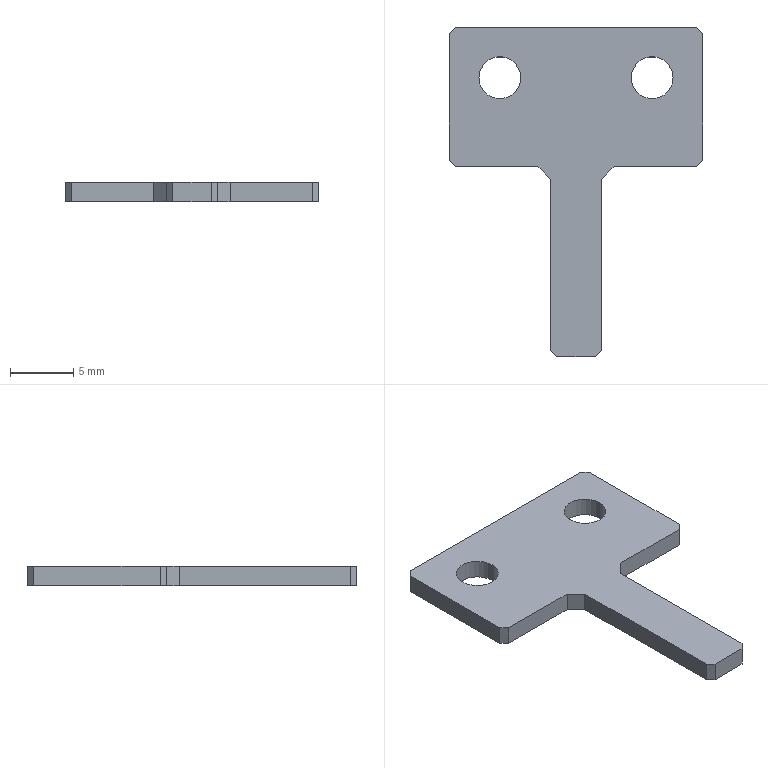Part | STEP file | 06-03 sensor plate | 1 solid | 22 faces | box 20 x 26 x 1.5 mm | volume 394.716 mm3 | plane 18 | cylinder 4 | commonest cylinder face diameters 3.3 x4
STEP:
#1=CARTESIAN_POINT('',(-4.35,9.,0.));
#2=VERTEX_POINT('',#1);
#3=CARTESIAN_POINT('',(-7.65,9.,0.));
#4=VERTEX_POINT('',#3);
#5=CARTESIAN_POINT('',(-6.,9.,0.));
#6=DIRECTION('',(0.,0.,-1.));
#7=DIRECTION('',(-1.,0.,0.));
#8=AXIS2_PLACEMENT_3D('',#5,#6,#7);
#9=CIRCLE('',#8,1.65);
#10=EDGE_CURVE('',#2,#4,#9,.T.);
#11=ORIENTED_EDGE('',*,*,#10,.T.);
#12=CARTESIAN_POINT('',(-7.65,9.,1.5));
#13=VERTEX_POINT('',#12);
#14=CARTESIAN_POINT('',(-7.65,9.,1.5));
#15=DIRECTION('',(0.,0.,1.));
#16=VECTOR('',#15,1000.);
#17=LINE('',#14,#16);
#18=EDGE_CURVE('',#4,#13,#17,.T.);
#19=ORIENTED_EDGE('',*,*,#18,.T.);
#20=CARTESIAN_POINT('',(-4.35,9.,1.5));
#21=VERTEX_POINT('',#20);
#22=CARTESIAN_POINT('',(-6.,9.,1.5));
#23=DIRECTION('',(0.,0.,1.));
#24=DIRECTION('',(1.,0.,0.));
#25=AXIS2_PLACEMENT_3D('',#22,#23,#24);
#26=CIRCLE('',#25,1.65);
#27=EDGE_CURVE('',#13,#21,#26,.T.);
#28=ORIENTED_EDGE('',*,*,#27,.T.);
#29=CARTESIAN_POINT('',(-4.35,9.,1.5));
#30=DIRECTION('',(0.,0.,1.));
#31=VECTOR('',#30,1000.);
#32=LINE('',#29,#31);
#33=EDGE_CURVE('',#2,#21,#32,.T.);
#34=ORIENTED_EDGE('',*,*,#33,.F.);
#35=EDGE_LOOP('',(#11,#19,#28,#34));
#36=FACE_OUTER_BOUND('',#35,.T.);
#37=CARTESIAN_POINT('',(-6.,9.,1.5));
#38=DIRECTION('',(0.,0.,1.));
#39=DIRECTION('',(1.,0.,0.));
#40=AXIS2_PLACEMENT_3D('',#37,#38,#39);
#41=CYLINDRICAL_SURFACE('',#40,1.65);
#42=ADVANCED_FACE('',(#36),#41,.F.);
#43=CARTESIAN_POINT('',(7.65,9.,0.));
#44=VERTEX_POINT('',#43);
#45=CARTESIAN_POINT('',(4.35,9.,0.));
#46=VERTEX_POINT('',#45);
#47=CARTESIAN_POINT('',(6.,9.,0.));
#48=DIRECTION('',(0.,0.,-1.));
#49=DIRECTION('',(-1.,0.,0.));
#50=AXIS2_PLACEMENT_3D('',#47,#48,#49);
#51=CIRCLE('',#50,1.65);
#52=EDGE_CURVE('',#44,#46,#51,.T.);
#53=ORIENTED_EDGE('',*,*,#52,.T.);
#54=CARTESIAN_POINT('',(4.35,9.,1.5));
#55=VERTEX_POINT('',#54);
#56=CARTESIAN_POINT('',(4.35,9.,1.5));
#57=DIRECTION('',(0.,0.,1.));
#58=VECTOR('',#57,1000.);
#59=LINE('',#56,#58);
#60=EDGE_CURVE('',#46,#55,#59,.T.);
#61=ORIENTED_EDGE('',*,*,#60,.T.);
#62=CARTESIAN_POINT('',(7.65,9.,1.5));
#63=VERTEX_POINT('',#62);
#64=CARTESIAN_POINT('',(6.,9.,1.5));
#65=DIRECTION('',(0.,0.,1.));
#66=DIRECTION('',(1.,0.,0.));
#67=AXIS2_PLACEMENT_3D('',#64,#65,#66);
#68=CIRCLE('',#67,1.65);
#69=EDGE_CURVE('',#55,#63,#68,.T.);
#70=ORIENTED_EDGE('',*,*,#69,.T.);
#71=CARTESIAN_POINT('',(7.65,9.,1.5));
#72=DIRECTION('',(0.,0.,1.));
#73=VECTOR('',#72,1000.);
#74=LINE('',#71,#73);
#75=EDGE_CURVE('',#44,#63,#74,.T.);
#76=ORIENTED_EDGE('',*,*,#75,.F.);
#77=EDGE_LOOP('',(#53,#61,#70,#76));
#78=FACE_OUTER_BOUND('',#77,.T.);
#79=CARTESIAN_POINT('',(6.,9.,1.5));
#80=DIRECTION('',(0.,0.,1.));
#81=DIRECTION('',(1.,0.,0.));
#82=AXIS2_PLACEMENT_3D('',#79,#80,#81);
#83=CYLINDRICAL_SURFACE('',#82,1.65);
#84=ADVANCED_FACE('',(#78),#83,.F.);
#85=CARTESIAN_POINT('',(10.,2.5,1.5));
#86=VERTEX_POINT('',#85);
#87=CARTESIAN_POINT('',(10.,12.5,1.5));
#88=VERTEX_POINT('',#87);
#89=CARTESIAN_POINT('',(10.,-13.,1.5));
#90=DIRECTION('',(0.,1.,0.));
#91=VECTOR('',#90,1000.);
#92=LINE('',#89,#91);
#93=EDGE_CURVE('',#86,#88,#92,.T.);
#94=ORIENTED_EDGE('',*,*,#93,.F.);
#95=CARTESIAN_POINT('',(10.,2.5,0.));
#96=VERTEX_POINT('',#95);
#97=CARTESIAN_POINT('',(10.,2.5,1.5));
#98=DIRECTION('',(0.,0.,-1.));
#99=VECTOR('',#98,1000.);
#100=LINE('',#97,#99);
#101=EDGE_CURVE('',#86,#96,#100,.T.);
#102=ORIENTED_EDGE('',*,*,#101,.T.);
#103=CARTESIAN_POINT('',(10.,12.5,0.));
#104=VERTEX_POINT('',#103);
#105=CARTESIAN_POINT('',(10.,-13.,0.));
#106=DIRECTION('',(0.,1.,0.));
#107=VECTOR('',#106,1000.);
#108=LINE('',#105,#107);
#109=EDGE_CURVE('',#96,#104,#108,.T.);
#110=ORIENTED_EDGE('',*,*,#109,.T.);
#111=CARTESIAN_POINT('',(10.,12.5,1.5));
#112=DIRECTION('',(0.,0.,1.));
#113=VECTOR('',#112,1000.);
#114=LINE('',#111,#113);
#115=EDGE_CURVE('',#104,#88,#114,.T.);
#116=ORIENTED_EDGE('',*,*,#115,.T.);
#117=EDGE_LOOP('',(#94,#102,#110,#116));
#118=FACE_OUTER_BOUND('',#117,.T.);
#119=CARTESIAN_POINT('',(10.,-13.,1.5));
#120=DIRECTION('',(-1.,0.,0.));
#121=DIRECTION('',(0.,0.,1.));
#122=AXIS2_PLACEMENT_3D('',#119,#120,#121);
#123=PLANE('',#122);
#124=ADVANCED_FACE('',(#118),#123,.F.);
#125=CARTESIAN_POINT('',(9.5,13.,1.5));
#126=VERTEX_POINT('',#125);
#127=CARTESIAN_POINT('',(-9.5,13.,1.5));
#128=VERTEX_POINT('',#127);
#129=CARTESIAN_POINT('',(-10.,13.,1.5));
#130=DIRECTION('',(-1.,0.,0.));
#131=VECTOR('',#130,1000.);
#132=LINE('',#129,#131);
#133=EDGE_CURVE('',#126,#128,#132,.T.);
#134=ORIENTED_EDGE('',*,*,#133,.F.);
#135=CARTESIAN_POINT('',(9.5,13.,0.));
#136=VERTEX_POINT('',#135);
#137=CARTESIAN_POINT('',(9.5,13.,1.5));
#138=DIRECTION('',(0.,0.,-1.));
#139=VECTOR('',#138,1000.);
#140=LINE('',#137,#139);
#141=EDGE_CURVE('',#126,#136,#140,.T.);
#142=ORIENTED_EDGE('',*,*,#141,.T.);
#143=CARTESIAN_POINT('',(-9.5,13.,0.));
#144=VERTEX_POINT('',#143);
#145=CARTESIAN_POINT('',(-10.,13.,0.));
#146=DIRECTION('',(-1.,0.,0.));
#147=VECTOR('',#146,1000.);
#148=LINE('',#145,#147);
#149=EDGE_CURVE('',#136,#144,#148,.T.);
#150=ORIENTED_EDGE('',*,*,#149,.T.);
#151=CARTESIAN_POINT('',(-9.5,13.,1.5));
#152=DIRECTION('',(0.,0.,1.));
#153=VECTOR('',#152,1000.);
#154=LINE('',#151,#153);
#155=EDGE_CURVE('',#144,#128,#154,.T.);
#156=ORIENTED_EDGE('',*,*,#155,.T.);
#157=EDGE_LOOP('',(#134,#142,#150,#156));
#158=FACE_OUTER_BOUND('',#157,.T.);
#159=CARTESIAN_POINT('',(-10.,13.,1.5));
#160=DIRECTION('',(0.,-1.,0.));
#161=DIRECTION('',(0.,0.,-1.));
#162=AXIS2_PLACEMENT_3D('',#159,#160,#161);
#163=PLANE('',#162);
#164=ADVANCED_FACE('',(#158),#163,.F.);
#165=CARTESIAN_POINT('',(-10.,12.5,0.));
#166=VERTEX_POINT('',#165);
#167=CARTESIAN_POINT('',(-10.,2.5,0.));
#168=VERTEX_POINT('',#167);
#169=CARTESIAN_POINT('',(-10.,-13.,0.));
#170=DIRECTION('',(0.,-1.,0.));
#171=VECTOR('',#170,1000.);
#172=LINE('',#169,#171);
#173=EDGE_CURVE('',#166,#168,#172,.T.);
#174=ORIENTED_EDGE('',*,*,#173,.T.);
#175=CARTESIAN_POINT('',(-10.,2.5,1.5));
#176=VERTEX_POINT('',#175);
#177=CARTESIAN_POINT('',(-10.,2.5,1.5));
#178=DIRECTION('',(0.,0.,1.));
#179=VECTOR('',#178,1000.);
#180=LINE('',#177,#179);
#181=EDGE_CURVE('',#168,#176,#180,.T.);
#182=ORIENTED_EDGE('',*,*,#181,.T.);
#183=CARTESIAN_POINT('',(-10.,12.5,1.5));
#184=VERTEX_POINT('',#183);
#185=CARTESIAN_POINT('',(-10.,-13.,1.5));
#186=DIRECTION('',(0.,-1.,0.));
#187=VECTOR('',#186,1000.);
#188=LINE('',#185,#187);
#189=EDGE_CURVE('',#184,#176,#188,.T.);
#190=ORIENTED_EDGE('',*,*,#189,.F.);
#191=CARTESIAN_POINT('',(-10.,12.5,1.5));
#192=DIRECTION('',(0.,0.,-1.));
#193=VECTOR('',#192,1000.);
#194=LINE('',#191,#193);
#195=EDGE_CURVE('',#184,#166,#194,.T.);
#196=ORIENTED_EDGE('',*,*,#195,.T.);
#197=EDGE_LOOP('',(#174,#182,#190,#196));
#198=FACE_OUTER_BOUND('',#197,.T.);
#199=CARTESIAN_POINT('',(-10.,-13.,1.5));
#200=DIRECTION('',(1.,0.,0.));
#201=DIRECTION('',(0.,0.,-1.));
#202=AXIS2_PLACEMENT_3D('',#199,#200,#201);
#203=PLANE('',#202);
#204=ADVANCED_FACE('',(#198),#203,.F.);
#205=CARTESIAN_POINT('',(-1.5,-13.,1.5));
#206=VERTEX_POINT('',#205);
#207=CARTESIAN_POINT('',(1.5,-13.,1.5));
#208=VERTEX_POINT('',#207);
#209=CARTESIAN_POINT('',(-10.,-13.,1.5));
#210=DIRECTION('',(1.,0.,0.));
#211=VECTOR('',#210,1000.);
#212=LINE('',#209,#211);
#213=EDGE_CURVE('',#206,#208,#212,.T.);
#214=ORIENTED_EDGE('',*,*,#213,.F.);
#215=CARTESIAN_POINT('',(-1.5,-13.,0.));
#216=VERTEX_POINT('',#215);
#217=CARTESIAN_POINT('',(-1.5,-13.,1.5));
#218=DIRECTION('',(0.,0.,-1.));
#219=VECTOR('',#218,1000.);
#220=LINE('',#217,#219);
#221=EDGE_CURVE('',#206,#216,#220,.T.);
#222=ORIENTED_EDGE('',*,*,#221,.T.);
#223=CARTESIAN_POINT('',(1.5,-13.,0.));
#224=VERTEX_POINT('',#223);
#225=CARTESIAN_POINT('',(-10.,-13.,0.));
#226=DIRECTION('',(1.,0.,0.));
#227=VECTOR('',#226,1000.);
#228=LINE('',#225,#227);
#229=EDGE_CURVE('',#216,#224,#228,.T.);
#230=ORIENTED_EDGE('',*,*,#229,.T.);
#231=CARTESIAN_POINT('',(1.5,-13.,1.5));
#232=DIRECTION('',(0.,0.,1.));
#233=VECTOR('',#232,1000.);
#234=LINE('',#231,#233);
#235=EDGE_CURVE('',#224,#208,#234,.T.);
#236=ORIENTED_EDGE('',*,*,#235,.T.);
#237=EDGE_LOOP('',(#214,#222,#230,#236));
#238=FACE_OUTER_BOUND('',#237,.T.);
#239=CARTESIAN_POINT('',(-10.,-13.,1.5));
#240=DIRECTION('',(0.,1.,0.));
#241=DIRECTION('',(0.,0.,1.));
#242=AXIS2_PLACEMENT_3D('',#239,#240,#241);
#243=PLANE('',#242);
#244=ADVANCED_FACE('',(#238),#243,.F.);
#245=CARTESIAN_POINT('',(-6.,9.,1.5));
#246=DIRECTION('',(0.,0.,1.));
#247=DIRECTION('',(1.,0.,0.));
#248=AXIS2_PLACEMENT_3D('',#245,#246,#247);
#249=CIRCLE('',#248,1.65);
#250=EDGE_CURVE('',#21,#13,#249,.T.);
#251=ORIENTED_EDGE('',*,*,#250,.F.);
#252=ORIENTED_EDGE('',*,*,#27,.F.);
#253=EDGE_LOOP('',(#251,#252));
#254=FACE_BOUND('',#253,.T.);
#255=CARTESIAN_POINT('',(6.,9.,1.5));
#256=DIRECTION('',(0.,0.,1.));
#257=DIRECTION('',(1.,0.,0.));
#258=AXIS2_PLACEMENT_3D('',#255,#256,#257);
#259=CIRCLE('',#258,1.65);
#260=EDGE_CURVE('',#63,#55,#259,.T.);
#261=ORIENTED_EDGE('',*,*,#260,.F.);
#262=ORIENTED_EDGE('',*,*,#69,.F.);
#263=EDGE_LOOP('',(#261,#262));
#264=FACE_BOUND('',#263,.T.);
#265=CARTESIAN_POINT('',(-2.,-12.5,1.5));
#266=VERTEX_POINT('',#265);
#267=CARTESIAN_POINT('',(-2.,1.,1.5));
#268=VERTEX_POINT('',#267);
#269=CARTESIAN_POINT('',(-2.,-13.,1.5));
#270=DIRECTION('',(0.,1.,0.));
#271=VECTOR('',#270,1000.);
#272=LINE('',#269,#271);
#273=EDGE_CURVE('',#266,#268,#272,.T.);
#274=ORIENTED_EDGE('',*,*,#273,.F.);
#275=CARTESIAN_POINT('',(-2.,-12.5,1.5));
#276=DIRECTION('',(0.7071,-0.7071,0.));
#277=VECTOR('',#276,1000.);
#278=LINE('',#275,#277);
#279=EDGE_CURVE('',#266,#206,#278,.T.);
#280=ORIENTED_EDGE('',*,*,#279,.T.);
#281=ORIENTED_EDGE('',*,*,#213,.T.);
#282=CARTESIAN_POINT('',(2.,-12.5,1.5));
#283=VERTEX_POINT('',#282);
#284=CARTESIAN_POINT('',(1.5,-13.,1.5));
#285=DIRECTION('',(0.7071,0.7071,0.));
#286=VECTOR('',#285,1000.);
#287=LINE('',#284,#286);
#288=EDGE_CURVE('',#208,#283,#287,.T.);
#289=ORIENTED_EDGE('',*,*,#288,.T.);
#290=CARTESIAN_POINT('',(2.,1.,1.5));
#291=VERTEX_POINT('',#290);
#292=CARTESIAN_POINT('',(2.,-13.,1.5));
#293=DIRECTION('',(0.,-1.,0.));
#294=VECTOR('',#293,1000.);
#295=LINE('',#292,#294);
#296=EDGE_CURVE('',#291,#283,#295,.T.);
#297=ORIENTED_EDGE('',*,*,#296,.F.);
#298=CARTESIAN_POINT('',(3.,2.,1.5));
#299=VERTEX_POINT('',#298);
#300=CARTESIAN_POINT('',(12.,11.,1.5));
#301=DIRECTION('',(0.7071,0.7071,0.));
#302=VECTOR('',#301,1000.);
#303=LINE('',#300,#302);
#304=EDGE_CURVE('',#291,#299,#303,.T.);
#305=ORIENTED_EDGE('',*,*,#304,.T.);
#306=CARTESIAN_POINT('',(9.5,2.,1.5));
#307=VERTEX_POINT('',#306);
#308=CARTESIAN_POINT('',(10.,2.,1.5));
#309=DIRECTION('',(-1.,0.,0.));
#310=VECTOR('',#309,1000.);
#311=LINE('',#308,#310);
#312=EDGE_CURVE('',#307,#299,#311,.T.);
#313=ORIENTED_EDGE('',*,*,#312,.F.);
#314=CARTESIAN_POINT('',(9.5,2.,1.5));
#315=DIRECTION('',(0.7071,0.7071,0.));
#316=VECTOR('',#315,1000.);
#317=LINE('',#314,#316);
#318=EDGE_CURVE('',#307,#86,#317,.T.);
#319=ORIENTED_EDGE('',*,*,#318,.T.);
#320=ORIENTED_EDGE('',*,*,#93,.T.);
#321=CARTESIAN_POINT('',(9.5,13.,1.5));
#322=DIRECTION('',(-0.7071,0.7071,0.));
#323=VECTOR('',#322,1000.);
#324=LINE('',#321,#323);
#325=EDGE_CURVE('',#88,#126,#324,.T.);
#326=ORIENTED_EDGE('',*,*,#325,.T.);
#327=ORIENTED_EDGE('',*,*,#133,.T.);
#328=CARTESIAN_POINT('',(-10.,12.5,1.5));
#329=DIRECTION('',(-0.7071,-0.7071,0.));
#330=VECTOR('',#329,1000.);
#331=LINE('',#328,#330);
#332=EDGE_CURVE('',#128,#184,#331,.T.);
#333=ORIENTED_EDGE('',*,*,#332,.T.);
#334=ORIENTED_EDGE('',*,*,#189,.T.);
#335=CARTESIAN_POINT('',(-9.5,2.,1.5));
#336=VERTEX_POINT('',#335);
#337=CARTESIAN_POINT('',(-10.,2.5,1.5));
#338=DIRECTION('',(0.7071,-0.7071,0.));
#339=VECTOR('',#338,1000.);
#340=LINE('',#337,#339);
#341=EDGE_CURVE('',#176,#336,#340,.T.);
#342=ORIENTED_EDGE('',*,*,#341,.T.);
#343=CARTESIAN_POINT('',(-3.,2.,1.5));
#344=VERTEX_POINT('',#343);
#345=CARTESIAN_POINT('',(-10.,2.,1.5));
#346=DIRECTION('',(-1.,0.,0.));
#347=VECTOR('',#346,1000.);
#348=LINE('',#345,#347);
#349=EDGE_CURVE('',#344,#336,#348,.T.);
#350=ORIENTED_EDGE('',*,*,#349,.F.);
#351=CARTESIAN_POINT('',(-2.,1.,1.5));
#352=DIRECTION('',(0.7071,-0.7071,0.));
#353=VECTOR('',#352,1000.);
#354=LINE('',#351,#353);
#355=EDGE_CURVE('',#344,#268,#354,.T.);
#356=ORIENTED_EDGE('',*,*,#355,.T.);
#357=EDGE_LOOP('',(#274,#280,#281,#289,#297,#305,#313,#319,#320,#326,#327,#333,#334,#342,#350,#356));
#358=FACE_OUTER_BOUND('',#357,.T.);
#359=CARTESIAN_POINT('',(10.,13.,1.5));
#360=DIRECTION('',(0.,0.,-1.));
#361=DIRECTION('',(-1.,0.,0.));
#362=AXIS2_PLACEMENT_3D('',#359,#360,#361);
#363=PLANE('',#362);
#364=ADVANCED_FACE('',(#254,#264,#358),#363,.F.);
#365=ORIENTED_EDGE('',*,*,#229,.F.);
#366=CARTESIAN_POINT('',(-2.,-12.5,0.));
#367=VERTEX_POINT('',#366);
#368=CARTESIAN_POINT('',(-8.75,-5.75,0.));
#369=DIRECTION('',(-0.7071,0.7071,0.));
#370=VECTOR('',#369,1000.);
#371=LINE('',#368,#370);
#372=EDGE_CURVE('',#216,#367,#371,.T.);
#373=ORIENTED_EDGE('',*,*,#372,.T.);
#374=CARTESIAN_POINT('',(-2.,1.,0.));
#375=VERTEX_POINT('',#374);
#376=CARTESIAN_POINT('',(-2.,-13.,0.));
#377=DIRECTION('',(0.,1.,0.));
#378=VECTOR('',#377,1000.);
#379=LINE('',#376,#378);
#380=EDGE_CURVE('',#367,#375,#379,.T.);
#381=ORIENTED_EDGE('',*,*,#380,.T.);
#382=CARTESIAN_POINT('',(-3.,2.,0.));
#383=VERTEX_POINT('',#382);
#384=CARTESIAN_POINT('',(-3.,2.,0.));
#385=DIRECTION('',(-0.7071,0.7071,0.));
#386=VECTOR('',#385,1000.);
#387=LINE('',#384,#386);
#388=EDGE_CURVE('',#375,#383,#387,.T.);
#389=ORIENTED_EDGE('',*,*,#388,.T.);
#390=CARTESIAN_POINT('',(-9.5,2.,0.));
#391=VERTEX_POINT('',#390);
#392=CARTESIAN_POINT('',(-10.,2.,0.));
#393=DIRECTION('',(-1.,0.,0.));
#394=VECTOR('',#393,1000.);
#395=LINE('',#392,#394);
#396=EDGE_CURVE('',#383,#391,#395,.T.);
#397=ORIENTED_EDGE('',*,*,#396,.T.);
#398=CARTESIAN_POINT('',(-5.25,-2.25,0.));
#399=DIRECTION('',(-0.7071,0.7071,0.));
#400=VECTOR('',#399,1000.);
#401=LINE('',#398,#400);
#402=EDGE_CURVE('',#391,#168,#401,.T.);
#403=ORIENTED_EDGE('',*,*,#402,.T.);
#404=ORIENTED_EDGE('',*,*,#173,.F.);
#405=CARTESIAN_POINT('',(0.25,22.75,0.));
#406=DIRECTION('',(0.7071,0.7071,0.));
#407=VECTOR('',#406,1000.);
#408=LINE('',#405,#407);
#409=EDGE_CURVE('',#166,#144,#408,.T.);
#410=ORIENTED_EDGE('',*,*,#409,.T.);
#411=ORIENTED_EDGE('',*,*,#149,.F.);
#412=CARTESIAN_POINT('',(9.75,12.75,0.));
#413=DIRECTION('',(0.7071,-0.7071,0.));
#414=VECTOR('',#413,1000.);
#415=LINE('',#412,#414);
#416=EDGE_CURVE('',#136,#104,#415,.T.);
#417=ORIENTED_EDGE('',*,*,#416,.T.);
#418=ORIENTED_EDGE('',*,*,#109,.F.);
#419=CARTESIAN_POINT('',(9.5,2.,0.));
#420=VERTEX_POINT('',#419);
#421=CARTESIAN_POINT('',(15.25,7.75,0.));
#422=DIRECTION('',(-0.7071,-0.7071,0.));
#423=VECTOR('',#422,1000.);
#424=LINE('',#421,#423);
#425=EDGE_CURVE('',#96,#420,#424,.T.);
#426=ORIENTED_EDGE('',*,*,#425,.T.);
#427=CARTESIAN_POINT('',(3.,2.,0.));
#428=VERTEX_POINT('',#427);
#429=CARTESIAN_POINT('',(10.,2.,0.));
#430=DIRECTION('',(-1.,0.,0.));
#431=VECTOR('',#430,1000.);
#432=LINE('',#429,#431);
#433=EDGE_CURVE('',#420,#428,#432,.T.);
#434=ORIENTED_EDGE('',*,*,#433,.T.);
#435=CARTESIAN_POINT('',(2.,1.,0.));
#436=VERTEX_POINT('',#435);
#437=CARTESIAN_POINT('',(2.,1.,0.));
#438=DIRECTION('',(-0.7071,-0.7071,0.));
#439=VECTOR('',#438,1000.);
#440=LINE('',#437,#439);
#441=EDGE_CURVE('',#428,#436,#440,.T.);
#442=ORIENTED_EDGE('',*,*,#441,.T.);
#443=CARTESIAN_POINT('',(2.,-12.5,0.));
#444=VERTEX_POINT('',#443);
#445=CARTESIAN_POINT('',(2.,-13.,0.));
#446=DIRECTION('',(0.,-1.,0.));
#447=VECTOR('',#446,1000.);
#448=LINE('',#445,#447);
#449=EDGE_CURVE('',#436,#444,#448,.T.);
#450=ORIENTED_EDGE('',*,*,#449,.T.);
#451=CARTESIAN_POINT('',(18.75,4.25,0.));
#452=DIRECTION('',(-0.7071,-0.7071,0.));
#453=VECTOR('',#452,1000.);
#454=LINE('',#451,#453);
#455=EDGE_CURVE('',#444,#224,#454,.T.);
#456=ORIENTED_EDGE('',*,*,#455,.T.);
#457=EDGE_LOOP('',(#365,#373,#381,#389,#397,#403,#404,#410,#411,#417,#418,#426,#434,#442,#450,#456));
#458=FACE_OUTER_BOUND('',#457,.T.);
#459=ORIENTED_EDGE('',*,*,#10,.F.);
#460=CARTESIAN_POINT('',(-6.,9.,0.));
#461=DIRECTION('',(0.,0.,-1.));
#462=DIRECTION('',(-1.,0.,0.));
#463=AXIS2_PLACEMENT_3D('',#460,#461,#462);
#464=CIRCLE('',#463,1.65);
#465=EDGE_CURVE('',#4,#2,#464,.T.);
#466=ORIENTED_EDGE('',*,*,#465,.F.);
#467=EDGE_LOOP('',(#459,#466));
#468=FACE_BOUND('',#467,.T.);
#469=ORIENTED_EDGE('',*,*,#52,.F.);
#470=CARTESIAN_POINT('',(6.,9.,0.));
#471=DIRECTION('',(0.,0.,-1.));
#472=DIRECTION('',(-1.,0.,0.));
#473=AXIS2_PLACEMENT_3D('',#470,#471,#472);
#474=CIRCLE('',#473,1.65);
#475=EDGE_CURVE('',#46,#44,#474,.T.);
#476=ORIENTED_EDGE('',*,*,#475,.F.);
#477=EDGE_LOOP('',(#469,#476));
#478=FACE_BOUND('',#477,.T.);
#479=CARTESIAN_POINT('',(10.,13.,0.));
#480=DIRECTION('',(0.,0.,-1.));
#481=DIRECTION('',(-1.,0.,0.));
#482=AXIS2_PLACEMENT_3D('',#479,#480,#481);
#483=PLANE('',#482);
#484=ADVANCED_FACE('',(#458,#468,#478),#483,.T.);
#485=ORIENTED_EDGE('',*,*,#60,.F.);
#486=ORIENTED_EDGE('',*,*,#475,.T.);
#487=ORIENTED_EDGE('',*,*,#75,.T.);
#488=ORIENTED_EDGE('',*,*,#260,.T.);
#489=EDGE_LOOP('',(#485,#486,#487,#488));
#490=FACE_OUTER_BOUND('',#489,.T.);
#491=CARTESIAN_POINT('',(6.,9.,1.5));
#492=DIRECTION('',(0.,0.,1.));
#493=DIRECTION('',(1.,0.,0.));
#494=AXIS2_PLACEMENT_3D('',#491,#492,#493);
#495=CYLINDRICAL_SURFACE('',#494,1.65);
#496=ADVANCED_FACE('',(#490),#495,.F.);
#497=ORIENTED_EDGE('',*,*,#18,.F.);
#498=ORIENTED_EDGE('',*,*,#465,.T.);
#499=ORIENTED_EDGE('',*,*,#33,.T.);
#500=ORIENTED_EDGE('',*,*,#250,.T.);
#501=EDGE_LOOP('',(#497,#498,#499,#500));
#502=FACE_OUTER_BOUND('',#501,.T.);
#503=CARTESIAN_POINT('',(-6.,9.,1.5));
#504=DIRECTION('',(0.,0.,1.));
#505=DIRECTION('',(1.,0.,0.));
#506=AXIS2_PLACEMENT_3D('',#503,#504,#505);
#507=CYLINDRICAL_SURFACE('',#506,1.65);
#508=ADVANCED_FACE('',(#502),#507,.F.);
#509=ORIENTED_EDGE('',*,*,#396,.F.);
#510=CARTESIAN_POINT('',(-3.,2.,1.5));
#511=DIRECTION('',(0.,0.,1.));
#512=VECTOR('',#511,1000.);
#513=LINE('',#510,#512);
#514=EDGE_CURVE('',#383,#344,#513,.T.);
#515=ORIENTED_EDGE('',*,*,#514,.T.);
#516=ORIENTED_EDGE('',*,*,#349,.T.);
#517=CARTESIAN_POINT('',(-9.5,2.,0.));
#518=DIRECTION('',(0.,0.,-1.));
#519=VECTOR('',#518,1000.);
#520=LINE('',#517,#519);
#521=EDGE_CURVE('',#336,#391,#520,.T.);
#522=ORIENTED_EDGE('',*,*,#521,.T.);
#523=EDGE_LOOP('',(#509,#515,#516,#522));
#524=FACE_OUTER_BOUND('',#523,.T.);
#525=CARTESIAN_POINT('',(-10.,2.,0.));
#526=DIRECTION('',(0.,1.,0.));
#527=DIRECTION('',(0.,0.,1.));
#528=AXIS2_PLACEMENT_3D('',#525,#526,#527);
#529=PLANE('',#528);
#530=ADVANCED_FACE('',(#524),#529,.F.);
#531=ORIENTED_EDGE('',*,*,#273,.T.);
#532=CARTESIAN_POINT('',(-2.,1.,0.));
#533=DIRECTION('',(0.,0.,-1.));
#534=VECTOR('',#533,1000.);
#535=LINE('',#532,#534);
#536=EDGE_CURVE('',#268,#375,#535,.T.);
#537=ORIENTED_EDGE('',*,*,#536,.T.);
#538=ORIENTED_EDGE('',*,*,#380,.F.);
#539=CARTESIAN_POINT('',(-2.,-12.5,0.));
#540=DIRECTION('',(0.,0.,1.));
#541=VECTOR('',#540,1000.);
#542=LINE('',#539,#541);
#543=EDGE_CURVE('',#367,#266,#542,.T.);
#544=ORIENTED_EDGE('',*,*,#543,.T.);
#545=EDGE_LOOP('',(#531,#537,#538,#544));
#546=FACE_OUTER_BOUND('',#545,.T.);
#547=CARTESIAN_POINT('',(-2.,-13.,0.));
#548=DIRECTION('',(1.,0.,0.));
#549=DIRECTION('',(0.,0.,-1.));
#550=AXIS2_PLACEMENT_3D('',#547,#548,#549);
#551=PLANE('',#550);
#552=ADVANCED_FACE('',(#546),#551,.F.);
#553=ORIENTED_EDGE('',*,*,#449,.F.);
#554=CARTESIAN_POINT('',(2.,1.,1.5));
#555=DIRECTION('',(0.,0.,1.));
#556=VECTOR('',#555,1000.);
#557=LINE('',#554,#556);
#558=EDGE_CURVE('',#436,#291,#557,.T.);
#559=ORIENTED_EDGE('',*,*,#558,.T.);
#560=ORIENTED_EDGE('',*,*,#296,.T.);
#561=CARTESIAN_POINT('',(2.,-12.5,0.));
#562=DIRECTION('',(0.,0.,-1.));
#563=VECTOR('',#562,1000.);
#564=LINE('',#561,#563);
#565=EDGE_CURVE('',#283,#444,#564,.T.);
#566=ORIENTED_EDGE('',*,*,#565,.T.);
#567=EDGE_LOOP('',(#553,#559,#560,#566));
#568=FACE_OUTER_BOUND('',#567,.T.);
#569=CARTESIAN_POINT('',(2.,-13.,0.));
#570=DIRECTION('',(-1.,0.,0.));
#571=DIRECTION('',(0.,0.,1.));
#572=AXIS2_PLACEMENT_3D('',#569,#570,#571);
#573=PLANE('',#572);
#574=ADVANCED_FACE('',(#568),#573,.F.);
#575=ORIENTED_EDGE('',*,*,#312,.T.);
#576=CARTESIAN_POINT('',(3.,2.,0.));
#577=DIRECTION('',(0.,0.,-1.));
#578=VECTOR('',#577,1000.);
#579=LINE('',#576,#578);
#580=EDGE_CURVE('',#299,#428,#579,.T.);
#581=ORIENTED_EDGE('',*,*,#580,.T.);
#582=ORIENTED_EDGE('',*,*,#433,.F.);
#583=CARTESIAN_POINT('',(9.5,2.,0.));
#584=DIRECTION('',(0.,0.,1.));
#585=VECTOR('',#584,1000.);
#586=LINE('',#583,#585);
#587=EDGE_CURVE('',#420,#307,#586,.T.);
#588=ORIENTED_EDGE('',*,*,#587,.T.);
#589=EDGE_LOOP('',(#575,#581,#582,#588));
#590=FACE_OUTER_BOUND('',#589,.T.);
#591=CARTESIAN_POINT('',(10.,2.,0.));
#592=DIRECTION('',(0.,1.,0.));
#593=DIRECTION('',(0.,0.,1.));
#594=AXIS2_PLACEMENT_3D('',#591,#592,#593);
#595=PLANE('',#594);
#596=ADVANCED_FACE('',(#590),#595,.F.);
#597=ORIENTED_EDGE('',*,*,#372,.F.);
#598=ORIENTED_EDGE('',*,*,#221,.F.);
#599=ORIENTED_EDGE('',*,*,#279,.F.);
#600=ORIENTED_EDGE('',*,*,#543,.F.);
#601=EDGE_LOOP('',(#597,#598,#599,#600));
#602=FACE_OUTER_BOUND('',#601,.T.);
#603=CARTESIAN_POINT('',(-2.,-12.5,0.));
#604=DIRECTION('',(0.7071,0.7071,0.));
#605=DIRECTION('',(-0.7071,0.7071,0.));
#606=AXIS2_PLACEMENT_3D('',#603,#604,#605);
#607=PLANE('',#606);
#608=ADVANCED_FACE('',(#602),#607,.F.);
#609=ORIENTED_EDGE('',*,*,#455,.F.);
#610=ORIENTED_EDGE('',*,*,#565,.F.);
#611=ORIENTED_EDGE('',*,*,#288,.F.);
#612=ORIENTED_EDGE('',*,*,#235,.F.);
#613=EDGE_LOOP('',(#609,#610,#611,#612));
#614=FACE_OUTER_BOUND('',#613,.T.);
#615=CARTESIAN_POINT('',(1.5,-13.,1.5));
#616=DIRECTION('',(-0.7071,0.7071,0.));
#617=DIRECTION('',(-0.7071,-0.7071,0.));
#618=AXIS2_PLACEMENT_3D('',#615,#616,#617);
#619=PLANE('',#618);
#620=ADVANCED_FACE('',(#614),#619,.F.);
#621=ORIENTED_EDGE('',*,*,#425,.F.);
#622=ORIENTED_EDGE('',*,*,#101,.F.);
#623=ORIENTED_EDGE('',*,*,#318,.F.);
#624=ORIENTED_EDGE('',*,*,#587,.F.);
#625=EDGE_LOOP('',(#621,#622,#623,#624));
#626=FACE_OUTER_BOUND('',#625,.T.);
#627=CARTESIAN_POINT('',(9.5,2.,0.));
#628=DIRECTION('',(-0.7071,0.7071,0.));
#629=DIRECTION('',(-0.7071,-0.7071,0.));
#630=AXIS2_PLACEMENT_3D('',#627,#628,#629);
#631=PLANE('',#630);
#632=ADVANCED_FACE('',(#626),#631,.F.);
#633=ORIENTED_EDGE('',*,*,#325,.F.);
#634=ORIENTED_EDGE('',*,*,#115,.F.);
#635=ORIENTED_EDGE('',*,*,#416,.F.);
#636=ORIENTED_EDGE('',*,*,#141,.F.);
#637=EDGE_LOOP('',(#633,#634,#635,#636));
#638=FACE_OUTER_BOUND('',#637,.T.);
#639=CARTESIAN_POINT('',(9.5,13.,1.5));
#640=DIRECTION('',(-0.7071,-0.7071,0.));
#641=DIRECTION('',(0.7071,-0.7071,0.));
#642=AXIS2_PLACEMENT_3D('',#639,#640,#641);
#643=PLANE('',#642);
#644=ADVANCED_FACE('',(#638),#643,.F.);
#645=ORIENTED_EDGE('',*,*,#402,.F.);
#646=ORIENTED_EDGE('',*,*,#521,.F.);
#647=ORIENTED_EDGE('',*,*,#341,.F.);
#648=ORIENTED_EDGE('',*,*,#181,.F.);
#649=EDGE_LOOP('',(#645,#646,#647,#648));
#650=FACE_OUTER_BOUND('',#649,.T.);
#651=CARTESIAN_POINT('',(-10.,2.5,1.5));
#652=DIRECTION('',(0.7071,0.7071,0.));
#653=DIRECTION('',(-0.7071,0.7071,0.));
#654=AXIS2_PLACEMENT_3D('',#651,#652,#653);
#655=PLANE('',#654);
#656=ADVANCED_FACE('',(#650),#655,.F.);
#657=ORIENTED_EDGE('',*,*,#332,.F.);
#658=ORIENTED_EDGE('',*,*,#155,.F.);
#659=ORIENTED_EDGE('',*,*,#409,.F.);
#660=ORIENTED_EDGE('',*,*,#195,.F.);
#661=EDGE_LOOP('',(#657,#658,#659,#660));
#662=FACE_OUTER_BOUND('',#661,.T.);
#663=CARTESIAN_POINT('',(-10.,12.5,1.5));
#664=DIRECTION('',(0.7071,-0.7071,0.));
#665=DIRECTION('',(0.7071,0.7071,0.));
#666=AXIS2_PLACEMENT_3D('',#663,#664,#665);
#667=PLANE('',#666);
#668=ADVANCED_FACE('',(#662),#667,.F.);
#669=ORIENTED_EDGE('',*,*,#441,.F.);
#670=ORIENTED_EDGE('',*,*,#580,.F.);
#671=ORIENTED_EDGE('',*,*,#304,.F.);
#672=ORIENTED_EDGE('',*,*,#558,.F.);
#673=EDGE_LOOP('',(#669,#670,#671,#672));
#674=FACE_OUTER_BOUND('',#673,.T.);
#675=CARTESIAN_POINT('',(2.,1.,0.));
#676=DIRECTION('',(0.7071,-0.7071,0.));
#677=DIRECTION('',(0.7071,0.7071,0.));
#678=AXIS2_PLACEMENT_3D('',#675,#676,#677);
#679=PLANE('',#678);
#680=ADVANCED_FACE('',(#674),#679,.T.);
#681=ORIENTED_EDGE('',*,*,#388,.F.);
#682=ORIENTED_EDGE('',*,*,#536,.F.);
#683=ORIENTED_EDGE('',*,*,#355,.F.);
#684=ORIENTED_EDGE('',*,*,#514,.F.);
#685=EDGE_LOOP('',(#681,#682,#683,#684));
#686=FACE_OUTER_BOUND('',#685,.T.);
#687=CARTESIAN_POINT('',(-3.,2.,0.));
#688=DIRECTION('',(-0.7071,-0.7071,0.));
#689=DIRECTION('',(0.7071,-0.7071,0.));
#690=AXIS2_PLACEMENT_3D('',#687,#688,#689);
#691=PLANE('',#690);
#692=ADVANCED_FACE('',(#686),#691,.T.);
#693=CLOSED_SHELL('',(#42,#84,#124,#164,#204,#244,#364,#484,#496,#508,#530,#552,#574,#596,#608,#620,#632,#644,#656,#668,#680,#692));
#694=MANIFOLD_SOLID_BREP('',#693);
#695=CARTESIAN_POINT('',(0.,0.,0.));
#696=DIRECTION('',(0.,0.,1.));
#697=DIRECTION('',(1.,0.,0.));
#698=AXIS2_PLACEMENT_3D('',#695,#696,#697);
#699=(LENGTH_UNIT()NAMED_UNIT(*)SI_UNIT(.MILLI.,.METRE.));
#700=UNCERTAINTY_MEASURE_WITH_UNIT(LENGTH_MEASURE(0.00001),#699,'','');
#701=(NAMED_UNIT(*)PLANE_ANGLE_UNIT()SI_UNIT($,.RADIAN.));
#702=(NAMED_UNIT(*)SI_UNIT($,.STERADIAN.)SOLID_ANGLE_UNIT());
#703=(GEOMETRIC_REPRESENTATION_CONTEXT(3)GLOBAL_UNCERTAINTY_ASSIGNED_CONTEXT((#700))GLOBAL_UNIT_ASSIGNED_CONTEXT((#699,#701,#702))REPRESENTATION_CONTEXT('',''));
#704=ADVANCED_BREP_SHAPE_REPRESENTATION('',(#694,#698),#703);